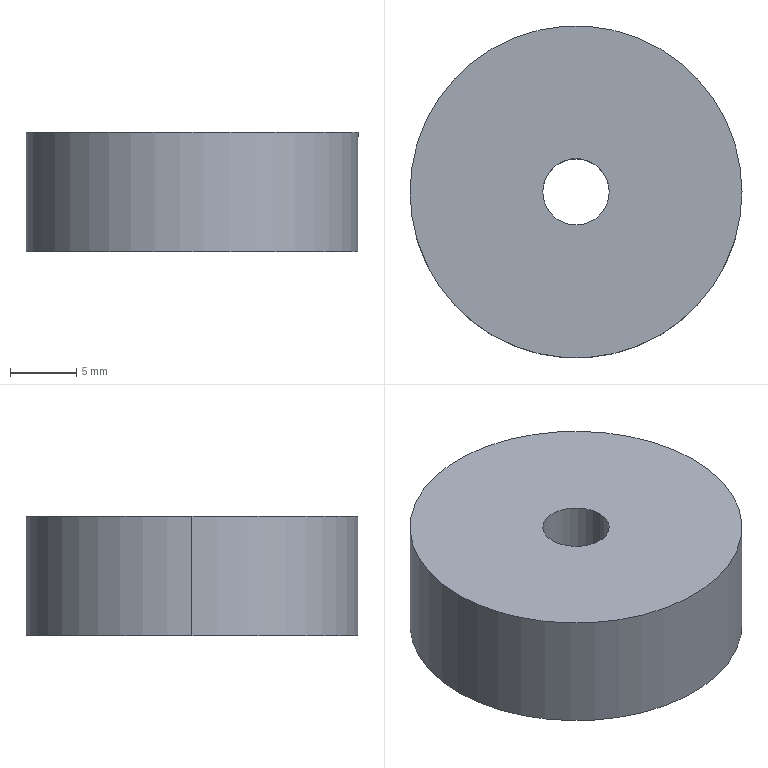Part | SolidWorks | features Revolution 1 | 1 solid | 6 faces | box 25 x 25 x 9 mm | volume 4241 mm3 | cylinder 4 | plane 2 | commonest cylinder face diameters 5 x2 25 x2
STEP:
#1=CARTESIAN_POINT('',(12.5,0.,-9.));
#2=VERTEX_POINT('',#1);
#3=CARTESIAN_POINT('',(-12.5,0.,-9.));
#4=VERTEX_POINT('',#3);
#5=CARTESIAN_POINT('',(0.,0.,-9.));
#6=DIRECTION('',(0.,0.,1.));
#7=DIRECTION('',(1.,0.,0.));
#8=AXIS2_PLACEMENT_3D('',#5,#6,#7);
#9=CIRCLE('',#8,12.5);
#10=EDGE_CURVE('',#2,#4,#9,.T.);
#11=ORIENTED_EDGE('',*,*,#10,.T.);
#12=CARTESIAN_POINT('',(-12.5,0.,0.));
#13=VERTEX_POINT('',#12);
#14=CARTESIAN_POINT('',(-12.5,0.,129.063));
#15=DIRECTION('',(0.,0.,1.));
#16=VECTOR('',#15,1000.);
#17=LINE('',#14,#16);
#18=EDGE_CURVE('',#4,#13,#17,.T.);
#19=ORIENTED_EDGE('',*,*,#18,.T.);
#20=CARTESIAN_POINT('',(12.5,0.,0.));
#21=VERTEX_POINT('',#20);
#22=CARTESIAN_POINT('',(0.,0.,0.));
#23=DIRECTION('',(0.,0.,1.));
#24=DIRECTION('',(1.,0.,0.));
#25=AXIS2_PLACEMENT_3D('',#22,#23,#24);
#26=CIRCLE('',#25,12.5);
#27=EDGE_CURVE('',#21,#13,#26,.T.);
#28=ORIENTED_EDGE('',*,*,#27,.F.);
#29=CARTESIAN_POINT('',(12.5,0.,129.063));
#30=DIRECTION('',(0.,0.,1.));
#31=VECTOR('',#30,1000.);
#32=LINE('',#29,#31);
#33=EDGE_CURVE('',#2,#21,#32,.T.);
#34=ORIENTED_EDGE('',*,*,#33,.F.);
#35=EDGE_LOOP('',(#11,#19,#28,#34));
#36=FACE_OUTER_BOUND('',#35,.T.);
#37=CARTESIAN_POINT('',(0.,0.,129.063));
#38=DIRECTION('',(0.,0.,1.));
#39=DIRECTION('',(1.,0.,0.));
#40=AXIS2_PLACEMENT_3D('',#37,#38,#39);
#41=CYLINDRICAL_SURFACE('',#40,12.5);
#42=ADVANCED_FACE('',(#36),#41,.T.);
#43=CARTESIAN_POINT('',(-2.5,0.,-9.));
#44=VERTEX_POINT('',#43);
#45=CARTESIAN_POINT('',(2.5,0.,-9.));
#46=VERTEX_POINT('',#45);
#47=CARTESIAN_POINT('',(0.,0.,-9.));
#48=DIRECTION('',(0.,0.,1.));
#49=DIRECTION('',(1.,0.,0.));
#50=AXIS2_PLACEMENT_3D('',#47,#48,#49);
#51=CIRCLE('',#50,2.5);
#52=EDGE_CURVE('',#44,#46,#51,.T.);
#53=ORIENTED_EDGE('',*,*,#52,.F.);
#54=CARTESIAN_POINT('',(-2.5,0.,0.));
#55=VERTEX_POINT('',#54);
#56=CARTESIAN_POINT('',(-2.5,0.,129.063));
#57=DIRECTION('',(0.,0.,1.));
#58=VECTOR('',#57,1000.);
#59=LINE('',#56,#58);
#60=EDGE_CURVE('',#44,#55,#59,.T.);
#61=ORIENTED_EDGE('',*,*,#60,.T.);
#62=CARTESIAN_POINT('',(2.5,0.,0.));
#63=VERTEX_POINT('',#62);
#64=CARTESIAN_POINT('',(0.,0.,0.));
#65=DIRECTION('',(0.,0.,1.));
#66=DIRECTION('',(1.,0.,0.));
#67=AXIS2_PLACEMENT_3D('',#64,#65,#66);
#68=CIRCLE('',#67,2.5);
#69=EDGE_CURVE('',#55,#63,#68,.T.);
#70=ORIENTED_EDGE('',*,*,#69,.T.);
#71=CARTESIAN_POINT('',(2.5,0.,129.063));
#72=DIRECTION('',(0.,0.,1.));
#73=VECTOR('',#72,1000.);
#74=LINE('',#71,#73);
#75=EDGE_CURVE('',#46,#63,#74,.T.);
#76=ORIENTED_EDGE('',*,*,#75,.F.);
#77=EDGE_LOOP('',(#53,#61,#70,#76));
#78=FACE_OUTER_BOUND('',#77,.T.);
#79=CARTESIAN_POINT('',(0.,0.,129.063));
#80=DIRECTION('',(0.,0.,1.));
#81=DIRECTION('',(1.,0.,0.));
#82=AXIS2_PLACEMENT_3D('',#79,#80,#81);
#83=CYLINDRICAL_SURFACE('',#82,2.5);
#84=ADVANCED_FACE('',(#78),#83,.F.);
#85=ORIENTED_EDGE('',*,*,#60,.F.);
#86=CARTESIAN_POINT('',(0.,0.,-9.));
#87=DIRECTION('',(0.,0.,1.));
#88=DIRECTION('',(1.,0.,0.));
#89=AXIS2_PLACEMENT_3D('',#86,#87,#88);
#90=CIRCLE('',#89,2.5);
#91=EDGE_CURVE('',#46,#44,#90,.T.);
#92=ORIENTED_EDGE('',*,*,#91,.F.);
#93=ORIENTED_EDGE('',*,*,#75,.T.);
#94=CARTESIAN_POINT('',(0.,0.,0.));
#95=DIRECTION('',(0.,0.,1.));
#96=DIRECTION('',(1.,0.,0.));
#97=AXIS2_PLACEMENT_3D('',#94,#95,#96);
#98=CIRCLE('',#97,2.5);
#99=EDGE_CURVE('',#63,#55,#98,.T.);
#100=ORIENTED_EDGE('',*,*,#99,.T.);
#101=EDGE_LOOP('',(#85,#92,#93,#100));
#102=FACE_OUTER_BOUND('',#101,.T.);
#103=CARTESIAN_POINT('',(0.,0.,129.063));
#104=DIRECTION('',(0.,0.,1.));
#105=DIRECTION('',(1.,0.,0.));
#106=AXIS2_PLACEMENT_3D('',#103,#104,#105);
#107=CYLINDRICAL_SURFACE('',#106,2.5);
#108=ADVANCED_FACE('',(#102),#107,.F.);
#109=ORIENTED_EDGE('',*,*,#99,.F.);
#110=ORIENTED_EDGE('',*,*,#69,.F.);
#111=EDGE_LOOP('',(#109,#110));
#112=FACE_BOUND('',#111,.T.);
#113=ORIENTED_EDGE('',*,*,#27,.T.);
#114=CARTESIAN_POINT('',(0.,0.,0.));
#115=DIRECTION('',(0.,0.,1.));
#116=DIRECTION('',(1.,0.,0.));
#117=AXIS2_PLACEMENT_3D('',#114,#115,#116);
#118=CIRCLE('',#117,12.5);
#119=EDGE_CURVE('',#13,#21,#118,.T.);
#120=ORIENTED_EDGE('',*,*,#119,.T.);
#121=EDGE_LOOP('',(#113,#120));
#122=FACE_OUTER_BOUND('',#121,.T.);
#123=CARTESIAN_POINT('',(-2.5,0.,0.));
#124=DIRECTION('',(0.,0.,-1.));
#125=DIRECTION('',(-1.,0.,0.));
#126=AXIS2_PLACEMENT_3D('',#123,#124,#125);
#127=PLANE('',#126);
#128=ADVANCED_FACE('',(#112,#122),#127,.F.);
#129=ORIENTED_EDGE('',*,*,#18,.F.);
#130=CARTESIAN_POINT('',(0.,0.,-9.));
#131=DIRECTION('',(0.,0.,1.));
#132=DIRECTION('',(1.,0.,0.));
#133=AXIS2_PLACEMENT_3D('',#130,#131,#132);
#134=CIRCLE('',#133,12.5);
#135=EDGE_CURVE('',#4,#2,#134,.T.);
#136=ORIENTED_EDGE('',*,*,#135,.T.);
#137=ORIENTED_EDGE('',*,*,#33,.T.);
#138=ORIENTED_EDGE('',*,*,#119,.F.);
#139=EDGE_LOOP('',(#129,#136,#137,#138));
#140=FACE_OUTER_BOUND('',#139,.T.);
#141=CARTESIAN_POINT('',(0.,0.,129.063));
#142=DIRECTION('',(0.,0.,1.));
#143=DIRECTION('',(1.,0.,0.));
#144=AXIS2_PLACEMENT_3D('',#141,#142,#143);
#145=CYLINDRICAL_SURFACE('',#144,12.5);
#146=ADVANCED_FACE('',(#140),#145,.T.);
#147=ORIENTED_EDGE('',*,*,#10,.F.);
#148=ORIENTED_EDGE('',*,*,#135,.F.);
#149=EDGE_LOOP('',(#147,#148));
#150=FACE_OUTER_BOUND('',#149,.T.);
#151=ORIENTED_EDGE('',*,*,#91,.T.);
#152=ORIENTED_EDGE('',*,*,#52,.T.);
#153=EDGE_LOOP('',(#151,#152));
#154=FACE_BOUND('',#153,.T.);
#155=CARTESIAN_POINT('',(-12.5,0.,-9.));
#156=DIRECTION('',(0.,0.,1.));
#157=DIRECTION('',(1.,0.,0.));
#158=AXIS2_PLACEMENT_3D('',#155,#156,#157);
#159=PLANE('',#158);
#160=ADVANCED_FACE('',(#150,#154),#159,.F.);
#161=CLOSED_SHELL('',(#42,#84,#108,#128,#146,#160));
#162=MANIFOLD_SOLID_BREP('',#161);
#163=CARTESIAN_POINT('',(0.,0.,0.));
#164=DIRECTION('',(0.,0.,1.));
#165=DIRECTION('',(1.,0.,0.));
#166=AXIS2_PLACEMENT_3D('',#163,#164,#165);
#167=(LENGTH_UNIT()NAMED_UNIT(*)SI_UNIT(.MILLI.,.METRE.));
#168=UNCERTAINTY_MEASURE_WITH_UNIT(LENGTH_MEASURE(0.00001),#167,'','');
#169=(NAMED_UNIT(*)PLANE_ANGLE_UNIT()SI_UNIT($,.RADIAN.));
#170=(NAMED_UNIT(*)SI_UNIT($,.STERADIAN.)SOLID_ANGLE_UNIT());
#171=(GEOMETRIC_REPRESENTATION_CONTEXT(3)GLOBAL_UNCERTAINTY_ASSIGNED_CONTEXT((#168))GLOBAL_UNIT_ASSIGNED_CONTEXT((#167,#169,#170))REPRESENTATION_CONTEXT('',''));
#172=ADVANCED_BREP_SHAPE_REPRESENTATION('',(#162,#166),#171);